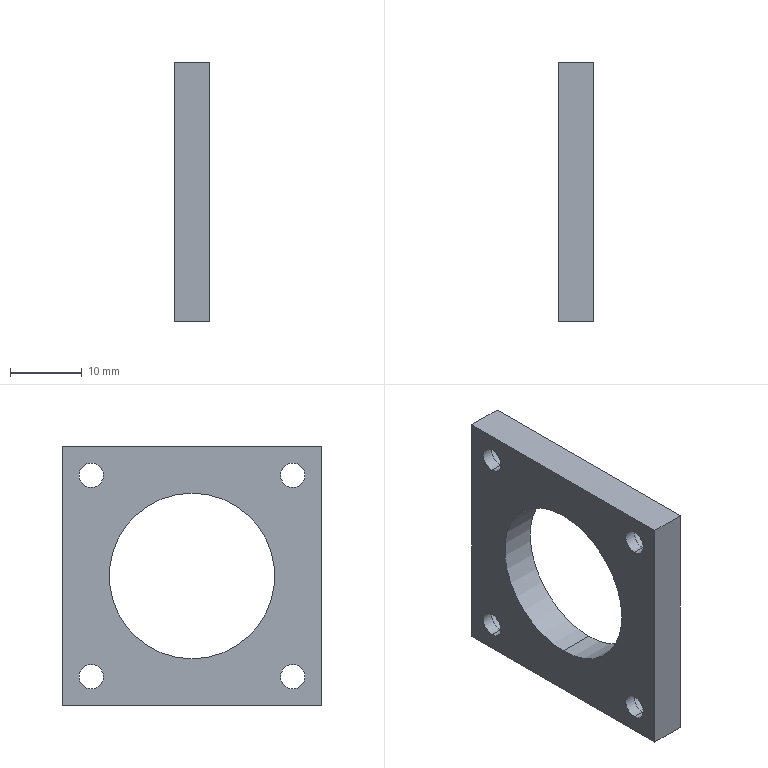Part | SolidWorks | features Extrusion 1, HoleWzd 1, ICE 1 | 1 solid | 28 faces | box 5 x 36 x 36 mm | volume 3893 mm3 | cylinder 18 | plane 10 | commonest cylinder face diameters 3.4 x8 6.5 x8 23 x2
STEP:
#1=CARTESIAN_POINT('',(-2.5,0.,11.5));
#2=VERTEX_POINT('',#1);
#3=CARTESIAN_POINT('',(-2.5,0.,-11.5));
#4=VERTEX_POINT('',#3);
#5=CARTESIAN_POINT('',(-2.5,0.,0.));
#6=DIRECTION('',(1.,0.,0.));
#7=DIRECTION('',(0.,0.,-1.));
#8=AXIS2_PLACEMENT_3D('',#5,#6,#7);
#9=CIRCLE('',#8,11.5);
#10=EDGE_CURVE('',#2,#4,#9,.T.);
#11=ORIENTED_EDGE('',*,*,#10,.F.);
#12=CARTESIAN_POINT('',(2.5,0.,11.5));
#13=VERTEX_POINT('',#12);
#14=CARTESIAN_POINT('',(-2.5,0.,11.5));
#15=DIRECTION('',(1.,0.,0.));
#16=VECTOR('',#15,1000.);
#17=LINE('',#14,#16);
#18=EDGE_CURVE('',#2,#13,#17,.T.);
#19=ORIENTED_EDGE('',*,*,#18,.T.);
#20=CARTESIAN_POINT('',(2.5,0.,-11.5));
#21=VERTEX_POINT('',#20);
#22=CARTESIAN_POINT('',(2.5,0.,0.));
#23=DIRECTION('',(1.,0.,0.));
#24=DIRECTION('',(0.,0.,-1.));
#25=AXIS2_PLACEMENT_3D('',#22,#23,#24);
#26=CIRCLE('',#25,11.5);
#27=EDGE_CURVE('',#13,#21,#26,.T.);
#28=ORIENTED_EDGE('',*,*,#27,.T.);
#29=CARTESIAN_POINT('',(-2.5,0.,-11.5));
#30=DIRECTION('',(1.,0.,0.));
#31=VECTOR('',#30,1000.);
#32=LINE('',#29,#31);
#33=EDGE_CURVE('',#4,#21,#32,.T.);
#34=ORIENTED_EDGE('',*,*,#33,.F.);
#35=EDGE_LOOP('',(#11,#19,#28,#34));
#36=FACE_OUTER_BOUND('',#35,.T.);
#37=CARTESIAN_POINT('',(-2.5,0.,0.));
#38=DIRECTION('',(1.,0.,0.));
#39=DIRECTION('',(0.,0.,-1.));
#40=AXIS2_PLACEMENT_3D('',#37,#38,#39);
#41=CYLINDRICAL_SURFACE('',#40,11.5);
#42=ADVANCED_FACE('',(#36),#41,.F.);
#43=CARTESIAN_POINT('',(-0.9,14.,17.25));
#44=VERTEX_POINT('',#43);
#45=CARTESIAN_POINT('',(-0.9,14.,10.75));
#46=VERTEX_POINT('',#45);
#47=CARTESIAN_POINT('',(-0.9,14.,14.));
#48=DIRECTION('',(1.,0.,0.));
#49=DIRECTION('',(0.,0.,-1.));
#50=AXIS2_PLACEMENT_3D('',#47,#48,#49);
#51=CIRCLE('',#50,3.25);
#52=EDGE_CURVE('',#44,#46,#51,.T.);
#53=ORIENTED_EDGE('',*,*,#52,.F.);
#54=CARTESIAN_POINT('',(2.5,14.,17.25));
#55=VERTEX_POINT('',#54);
#56=CARTESIAN_POINT('',(2.5,14.,17.25));
#57=DIRECTION('',(1.,0.,0.));
#58=VECTOR('',#57,1000.);
#59=LINE('',#56,#58);
#60=EDGE_CURVE('',#44,#55,#59,.T.);
#61=ORIENTED_EDGE('',*,*,#60,.T.);
#62=CARTESIAN_POINT('',(2.5,14.,10.75));
#63=VERTEX_POINT('',#62);
#64=CARTESIAN_POINT('',(2.5,14.,14.));
#65=DIRECTION('',(1.,0.,0.));
#66=DIRECTION('',(0.,0.,-1.));
#67=AXIS2_PLACEMENT_3D('',#64,#65,#66);
#68=CIRCLE('',#67,3.25);
#69=EDGE_CURVE('',#55,#63,#68,.T.);
#70=ORIENTED_EDGE('',*,*,#69,.T.);
#71=CARTESIAN_POINT('',(2.5,14.,10.75));
#72=DIRECTION('',(1.,0.,0.));
#73=VECTOR('',#72,1000.);
#74=LINE('',#71,#73);
#75=EDGE_CURVE('',#46,#63,#74,.T.);
#76=ORIENTED_EDGE('',*,*,#75,.F.);
#77=EDGE_LOOP('',(#53,#61,#70,#76));
#78=FACE_OUTER_BOUND('',#77,.T.);
#79=CARTESIAN_POINT('',(2.5,14.,14.));
#80=DIRECTION('',(1.,0.,0.));
#81=DIRECTION('',(0.,0.,-1.));
#82=AXIS2_PLACEMENT_3D('',#79,#80,#81);
#83=CYLINDRICAL_SURFACE('',#82,3.25);
#84=ADVANCED_FACE('',(#78),#83,.F.);
#85=CARTESIAN_POINT('',(-2.5,14.,15.7));
#86=VERTEX_POINT('',#85);
#87=CARTESIAN_POINT('',(-2.5,14.,12.3));
#88=VERTEX_POINT('',#87);
#89=CARTESIAN_POINT('',(-2.5,14.,14.));
#90=DIRECTION('',(1.,0.,0.));
#91=DIRECTION('',(0.,0.,-1.));
#92=AXIS2_PLACEMENT_3D('',#89,#90,#91);
#93=CIRCLE('',#92,1.7);
#94=EDGE_CURVE('',#86,#88,#93,.T.);
#95=ORIENTED_EDGE('',*,*,#94,.F.);
#96=CARTESIAN_POINT('',(-0.9,14.,15.7));
#97=VERTEX_POINT('',#96);
#98=CARTESIAN_POINT('',(2.5,14.,15.7));
#99=DIRECTION('',(1.,0.,0.));
#100=VECTOR('',#99,1000.);
#101=LINE('',#98,#100);
#102=EDGE_CURVE('',#86,#97,#101,.T.);
#103=ORIENTED_EDGE('',*,*,#102,.T.);
#104=CARTESIAN_POINT('',(-0.9,14.,12.3));
#105=VERTEX_POINT('',#104);
#106=CARTESIAN_POINT('',(-0.9,14.,14.));
#107=DIRECTION('',(1.,0.,0.));
#108=DIRECTION('',(0.,0.,-1.));
#109=AXIS2_PLACEMENT_3D('',#106,#107,#108);
#110=CIRCLE('',#109,1.7);
#111=EDGE_CURVE('',#97,#105,#110,.T.);
#112=ORIENTED_EDGE('',*,*,#111,.T.);
#113=CARTESIAN_POINT('',(2.5,14.,12.3));
#114=DIRECTION('',(1.,0.,0.));
#115=VECTOR('',#114,1000.);
#116=LINE('',#113,#115);
#117=EDGE_CURVE('',#88,#105,#116,.T.);
#118=ORIENTED_EDGE('',*,*,#117,.F.);
#119=EDGE_LOOP('',(#95,#103,#112,#118));
#120=FACE_OUTER_BOUND('',#119,.T.);
#121=CARTESIAN_POINT('',(2.5,14.,14.));
#122=DIRECTION('',(1.,0.,0.));
#123=DIRECTION('',(0.,0.,-1.));
#124=AXIS2_PLACEMENT_3D('',#121,#122,#123);
#125=CYLINDRICAL_SURFACE('',#124,1.7);
#126=ADVANCED_FACE('',(#120),#125,.F.);
#127=CARTESIAN_POINT('',(-0.9,14.,-10.75));
#128=VERTEX_POINT('',#127);
#129=CARTESIAN_POINT('',(-0.9,14.,-17.25));
#130=VERTEX_POINT('',#129);
#131=CARTESIAN_POINT('',(-0.9,14.,-14.));
#132=DIRECTION('',(1.,0.,0.));
#133=DIRECTION('',(0.,0.,-1.));
#134=AXIS2_PLACEMENT_3D('',#131,#132,#133);
#135=CIRCLE('',#134,3.25);
#136=EDGE_CURVE('',#128,#130,#135,.T.);
#137=ORIENTED_EDGE('',*,*,#136,.F.);
#138=CARTESIAN_POINT('',(2.5,14.,-10.75));
#139=VERTEX_POINT('',#138);
#140=CARTESIAN_POINT('',(2.5,14.,-10.75));
#141=DIRECTION('',(1.,0.,0.));
#142=VECTOR('',#141,1000.);
#143=LINE('',#140,#142);
#144=EDGE_CURVE('',#128,#139,#143,.T.);
#145=ORIENTED_EDGE('',*,*,#144,.T.);
#146=CARTESIAN_POINT('',(2.5,14.,-17.25));
#147=VERTEX_POINT('',#146);
#148=CARTESIAN_POINT('',(2.5,14.,-14.));
#149=DIRECTION('',(1.,0.,0.));
#150=DIRECTION('',(0.,0.,-1.));
#151=AXIS2_PLACEMENT_3D('',#148,#149,#150);
#152=CIRCLE('',#151,3.25);
#153=EDGE_CURVE('',#139,#147,#152,.T.);
#154=ORIENTED_EDGE('',*,*,#153,.T.);
#155=CARTESIAN_POINT('',(2.5,14.,-17.25));
#156=DIRECTION('',(1.,0.,0.));
#157=VECTOR('',#156,1000.);
#158=LINE('',#155,#157);
#159=EDGE_CURVE('',#130,#147,#158,.T.);
#160=ORIENTED_EDGE('',*,*,#159,.F.);
#161=EDGE_LOOP('',(#137,#145,#154,#160));
#162=FACE_OUTER_BOUND('',#161,.T.);
#163=CARTESIAN_POINT('',(2.5,14.,-14.));
#164=DIRECTION('',(1.,0.,0.));
#165=DIRECTION('',(0.,0.,-1.));
#166=AXIS2_PLACEMENT_3D('',#163,#164,#165);
#167=CYLINDRICAL_SURFACE('',#166,3.25);
#168=ADVANCED_FACE('',(#162),#167,.F.);
#169=CARTESIAN_POINT('',(-2.5,14.,-12.3));
#170=VERTEX_POINT('',#169);
#171=CARTESIAN_POINT('',(-2.5,14.,-15.7));
#172=VERTEX_POINT('',#171);
#173=CARTESIAN_POINT('',(-2.5,14.,-14.));
#174=DIRECTION('',(1.,0.,0.));
#175=DIRECTION('',(0.,0.,-1.));
#176=AXIS2_PLACEMENT_3D('',#173,#174,#175);
#177=CIRCLE('',#176,1.7);
#178=EDGE_CURVE('',#170,#172,#177,.T.);
#179=ORIENTED_EDGE('',*,*,#178,.F.);
#180=CARTESIAN_POINT('',(-0.9,14.,-12.3));
#181=VERTEX_POINT('',#180);
#182=CARTESIAN_POINT('',(2.5,14.,-12.3));
#183=DIRECTION('',(1.,0.,0.));
#184=VECTOR('',#183,1000.);
#185=LINE('',#182,#184);
#186=EDGE_CURVE('',#170,#181,#185,.T.);
#187=ORIENTED_EDGE('',*,*,#186,.T.);
#188=CARTESIAN_POINT('',(-0.9,14.,-15.7));
#189=VERTEX_POINT('',#188);
#190=CARTESIAN_POINT('',(-0.9,14.,-14.));
#191=DIRECTION('',(1.,0.,0.));
#192=DIRECTION('',(0.,0.,-1.));
#193=AXIS2_PLACEMENT_3D('',#190,#191,#192);
#194=CIRCLE('',#193,1.7);
#195=EDGE_CURVE('',#181,#189,#194,.T.);
#196=ORIENTED_EDGE('',*,*,#195,.T.);
#197=CARTESIAN_POINT('',(2.5,14.,-15.7));
#198=DIRECTION('',(1.,0.,0.));
#199=VECTOR('',#198,1000.);
#200=LINE('',#197,#199);
#201=EDGE_CURVE('',#172,#189,#200,.T.);
#202=ORIENTED_EDGE('',*,*,#201,.F.);
#203=EDGE_LOOP('',(#179,#187,#196,#202));
#204=FACE_OUTER_BOUND('',#203,.T.);
#205=CARTESIAN_POINT('',(2.5,14.,-14.));
#206=DIRECTION('',(1.,0.,0.));
#207=DIRECTION('',(0.,0.,-1.));
#208=AXIS2_PLACEMENT_3D('',#205,#206,#207);
#209=CYLINDRICAL_SURFACE('',#208,1.7);
#210=ADVANCED_FACE('',(#204),#209,.F.);
#211=CARTESIAN_POINT('',(-0.9,-14.,17.25));
#212=VERTEX_POINT('',#211);
#213=CARTESIAN_POINT('',(-0.9,-14.,10.75));
#214=VERTEX_POINT('',#213);
#215=CARTESIAN_POINT('',(-0.9,-14.,14.));
#216=DIRECTION('',(1.,0.,0.));
#217=DIRECTION('',(0.,0.,-1.));
#218=AXIS2_PLACEMENT_3D('',#215,#216,#217);
#219=CIRCLE('',#218,3.25);
#220=EDGE_CURVE('',#212,#214,#219,.T.);
#221=ORIENTED_EDGE('',*,*,#220,.F.);
#222=CARTESIAN_POINT('',(2.5,-14.,17.25));
#223=VERTEX_POINT('',#222);
#224=CARTESIAN_POINT('',(2.5,-14.,17.25));
#225=DIRECTION('',(1.,0.,0.));
#226=VECTOR('',#225,1000.);
#227=LINE('',#224,#226);
#228=EDGE_CURVE('',#212,#223,#227,.T.);
#229=ORIENTED_EDGE('',*,*,#228,.T.);
#230=CARTESIAN_POINT('',(2.5,-14.,10.75));
#231=VERTEX_POINT('',#230);
#232=CARTESIAN_POINT('',(2.5,-14.,14.));
#233=DIRECTION('',(1.,0.,0.));
#234=DIRECTION('',(0.,0.,-1.));
#235=AXIS2_PLACEMENT_3D('',#232,#233,#234);
#236=CIRCLE('',#235,3.25);
#237=EDGE_CURVE('',#223,#231,#236,.T.);
#238=ORIENTED_EDGE('',*,*,#237,.T.);
#239=CARTESIAN_POINT('',(2.5,-14.,10.75));
#240=DIRECTION('',(1.,0.,0.));
#241=VECTOR('',#240,1000.);
#242=LINE('',#239,#241);
#243=EDGE_CURVE('',#214,#231,#242,.T.);
#244=ORIENTED_EDGE('',*,*,#243,.F.);
#245=EDGE_LOOP('',(#221,#229,#238,#244));
#246=FACE_OUTER_BOUND('',#245,.T.);
#247=CARTESIAN_POINT('',(2.5,-14.,14.));
#248=DIRECTION('',(1.,0.,0.));
#249=DIRECTION('',(0.,0.,-1.));
#250=AXIS2_PLACEMENT_3D('',#247,#248,#249);
#251=CYLINDRICAL_SURFACE('',#250,3.25);
#252=ADVANCED_FACE('',(#246),#251,.F.);
#253=CARTESIAN_POINT('',(-2.5,-14.,15.7));
#254=VERTEX_POINT('',#253);
#255=CARTESIAN_POINT('',(-2.5,-14.,12.3));
#256=VERTEX_POINT('',#255);
#257=CARTESIAN_POINT('',(-2.5,-14.,14.));
#258=DIRECTION('',(1.,0.,0.));
#259=DIRECTION('',(0.,0.,-1.));
#260=AXIS2_PLACEMENT_3D('',#257,#258,#259);
#261=CIRCLE('',#260,1.7);
#262=EDGE_CURVE('',#254,#256,#261,.T.);
#263=ORIENTED_EDGE('',*,*,#262,.F.);
#264=CARTESIAN_POINT('',(-0.9,-14.,15.7));
#265=VERTEX_POINT('',#264);
#266=CARTESIAN_POINT('',(2.5,-14.,15.7));
#267=DIRECTION('',(1.,0.,0.));
#268=VECTOR('',#267,1000.);
#269=LINE('',#266,#268);
#270=EDGE_CURVE('',#254,#265,#269,.T.);
#271=ORIENTED_EDGE('',*,*,#270,.T.);
#272=CARTESIAN_POINT('',(-0.9,-14.,12.3));
#273=VERTEX_POINT('',#272);
#274=CARTESIAN_POINT('',(-0.9,-14.,14.));
#275=DIRECTION('',(1.,0.,0.));
#276=DIRECTION('',(0.,0.,-1.));
#277=AXIS2_PLACEMENT_3D('',#274,#275,#276);
#278=CIRCLE('',#277,1.7);
#279=EDGE_CURVE('',#265,#273,#278,.T.);
#280=ORIENTED_EDGE('',*,*,#279,.T.);
#281=CARTESIAN_POINT('',(2.5,-14.,12.3));
#282=DIRECTION('',(1.,0.,0.));
#283=VECTOR('',#282,1000.);
#284=LINE('',#281,#283);
#285=EDGE_CURVE('',#256,#273,#284,.T.);
#286=ORIENTED_EDGE('',*,*,#285,.F.);
#287=EDGE_LOOP('',(#263,#271,#280,#286));
#288=FACE_OUTER_BOUND('',#287,.T.);
#289=CARTESIAN_POINT('',(2.5,-14.,14.));
#290=DIRECTION('',(1.,0.,0.));
#291=DIRECTION('',(0.,0.,-1.));
#292=AXIS2_PLACEMENT_3D('',#289,#290,#291);
#293=CYLINDRICAL_SURFACE('',#292,1.7);
#294=ADVANCED_FACE('',(#288),#293,.F.);
#295=CARTESIAN_POINT('',(-0.9,-14.,-10.75));
#296=VERTEX_POINT('',#295);
#297=CARTESIAN_POINT('',(-0.9,-14.,-17.25));
#298=VERTEX_POINT('',#297);
#299=CARTESIAN_POINT('',(-0.9,-14.,-14.));
#300=DIRECTION('',(1.,0.,0.));
#301=DIRECTION('',(0.,0.,-1.));
#302=AXIS2_PLACEMENT_3D('',#299,#300,#301);
#303=CIRCLE('',#302,3.25);
#304=EDGE_CURVE('',#296,#298,#303,.T.);
#305=ORIENTED_EDGE('',*,*,#304,.F.);
#306=CARTESIAN_POINT('',(2.5,-14.,-10.75));
#307=VERTEX_POINT('',#306);
#308=CARTESIAN_POINT('',(2.5,-14.,-10.75));
#309=DIRECTION('',(1.,0.,0.));
#310=VECTOR('',#309,1000.);
#311=LINE('',#308,#310);
#312=EDGE_CURVE('',#296,#307,#311,.T.);
#313=ORIENTED_EDGE('',*,*,#312,.T.);
#314=CARTESIAN_POINT('',(2.5,-14.,-17.25));
#315=VERTEX_POINT('',#314);
#316=CARTESIAN_POINT('',(2.5,-14.,-14.));
#317=DIRECTION('',(1.,0.,0.));
#318=DIRECTION('',(0.,0.,-1.));
#319=AXIS2_PLACEMENT_3D('',#316,#317,#318);
#320=CIRCLE('',#319,3.25);
#321=EDGE_CURVE('',#307,#315,#320,.T.);
#322=ORIENTED_EDGE('',*,*,#321,.T.);
#323=CARTESIAN_POINT('',(2.5,-14.,-17.25));
#324=DIRECTION('',(1.,0.,0.));
#325=VECTOR('',#324,1000.);
#326=LINE('',#323,#325);
#327=EDGE_CURVE('',#298,#315,#326,.T.);
#328=ORIENTED_EDGE('',*,*,#327,.F.);
#329=EDGE_LOOP('',(#305,#313,#322,#328));
#330=FACE_OUTER_BOUND('',#329,.T.);
#331=CARTESIAN_POINT('',(2.5,-14.,-14.));
#332=DIRECTION('',(1.,0.,0.));
#333=DIRECTION('',(0.,0.,-1.));
#334=AXIS2_PLACEMENT_3D('',#331,#332,#333);
#335=CYLINDRICAL_SURFACE('',#334,3.25);
#336=ADVANCED_FACE('',(#330),#335,.F.);
#337=CARTESIAN_POINT('',(-2.5,-14.,-12.3));
#338=VERTEX_POINT('',#337);
#339=CARTESIAN_POINT('',(-2.5,-14.,-15.7));
#340=VERTEX_POINT('',#339);
#341=CARTESIAN_POINT('',(-2.5,-14.,-14.));
#342=DIRECTION('',(1.,0.,0.));
#343=DIRECTION('',(0.,0.,-1.));
#344=AXIS2_PLACEMENT_3D('',#341,#342,#343);
#345=CIRCLE('',#344,1.7);
#346=EDGE_CURVE('',#338,#340,#345,.T.);
#347=ORIENTED_EDGE('',*,*,#346,.F.);
#348=CARTESIAN_POINT('',(-0.9,-14.,-12.3));
#349=VERTEX_POINT('',#348);
#350=CARTESIAN_POINT('',(2.5,-14.,-12.3));
#351=DIRECTION('',(1.,0.,0.));
#352=VECTOR('',#351,1000.);
#353=LINE('',#350,#352);
#354=EDGE_CURVE('',#338,#349,#353,.T.);
#355=ORIENTED_EDGE('',*,*,#354,.T.);
#356=CARTESIAN_POINT('',(-0.9,-14.,-15.7));
#357=VERTEX_POINT('',#356);
#358=CARTESIAN_POINT('',(-0.9,-14.,-14.));
#359=DIRECTION('',(1.,0.,0.));
#360=DIRECTION('',(0.,0.,-1.));
#361=AXIS2_PLACEMENT_3D('',#358,#359,#360);
#362=CIRCLE('',#361,1.7);
#363=EDGE_CURVE('',#349,#357,#362,.T.);
#364=ORIENTED_EDGE('',*,*,#363,.T.);
#365=CARTESIAN_POINT('',(2.5,-14.,-15.7));
#366=DIRECTION('',(1.,0.,0.));
#367=VECTOR('',#366,1000.);
#368=LINE('',#365,#367);
#369=EDGE_CURVE('',#340,#357,#368,.T.);
#370=ORIENTED_EDGE('',*,*,#369,.F.);
#371=EDGE_LOOP('',(#347,#355,#364,#370));
#372=FACE_OUTER_BOUND('',#371,.T.);
#373=CARTESIAN_POINT('',(2.5,-14.,-14.));
#374=DIRECTION('',(1.,0.,0.));
#375=DIRECTION('',(0.,0.,-1.));
#376=AXIS2_PLACEMENT_3D('',#373,#374,#375);
#377=CYLINDRICAL_SURFACE('',#376,1.7);
#378=ADVANCED_FACE('',(#372),#377,.F.);
#379=CARTESIAN_POINT('',(-2.5,-18.,-18.));
#380=VERTEX_POINT('',#379);
#381=CARTESIAN_POINT('',(-2.5,18.,-18.));
#382=VERTEX_POINT('',#381);
#383=CARTESIAN_POINT('',(-2.5,18.,-18.));
#384=DIRECTION('',(0.,1.,0.));
#385=VECTOR('',#384,1000.);
#386=LINE('',#383,#385);
#387=EDGE_CURVE('',#380,#382,#386,.T.);
#388=ORIENTED_EDGE('',*,*,#387,.T.);
#389=CARTESIAN_POINT('',(2.5,18.,-18.));
#390=VERTEX_POINT('',#389);
#391=CARTESIAN_POINT('',(2.5,18.,-18.));
#392=DIRECTION('',(-1.,0.,0.));
#393=VECTOR('',#392,1000.);
#394=LINE('',#391,#393);
#395=EDGE_CURVE('',#390,#382,#394,.T.);
#396=ORIENTED_EDGE('',*,*,#395,.F.);
#397=CARTESIAN_POINT('',(2.5,-18.,-18.));
#398=VERTEX_POINT('',#397);
#399=CARTESIAN_POINT('',(2.5,18.,-18.));
#400=DIRECTION('',(0.,1.,0.));
#401=VECTOR('',#400,1000.);
#402=LINE('',#399,#401);
#403=EDGE_CURVE('',#398,#390,#402,.T.);
#404=ORIENTED_EDGE('',*,*,#403,.F.);
#405=CARTESIAN_POINT('',(2.5,-18.,-18.));
#406=DIRECTION('',(-1.,0.,0.));
#407=VECTOR('',#406,1000.);
#408=LINE('',#405,#407);
#409=EDGE_CURVE('',#398,#380,#408,.T.);
#410=ORIENTED_EDGE('',*,*,#409,.T.);
#411=EDGE_LOOP('',(#388,#396,#404,#410));
#412=FACE_OUTER_BOUND('',#411,.T.);
#413=CARTESIAN_POINT('',(2.5,18.,-18.));
#414=DIRECTION('',(0.,0.,1.));
#415=DIRECTION('',(0.,-1.,0.));
#416=AXIS2_PLACEMENT_3D('',#413,#414,#415);
#417=PLANE('',#416);
#418=ADVANCED_FACE('',(#412),#417,.F.);
#419=CARTESIAN_POINT('',(-2.5,18.,18.));
#420=VERTEX_POINT('',#419);
#421=CARTESIAN_POINT('',(-2.5,18.,18.));
#422=DIRECTION('',(0.,0.,1.));
#423=VECTOR('',#422,1000.);
#424=LINE('',#421,#423);
#425=EDGE_CURVE('',#382,#420,#424,.T.);
#426=ORIENTED_EDGE('',*,*,#425,.T.);
#427=CARTESIAN_POINT('',(2.5,18.,18.));
#428=VERTEX_POINT('',#427);
#429=CARTESIAN_POINT('',(2.5,18.,18.));
#430=DIRECTION('',(-1.,0.,0.));
#431=VECTOR('',#430,1000.);
#432=LINE('',#429,#431);
#433=EDGE_CURVE('',#428,#420,#432,.T.);
#434=ORIENTED_EDGE('',*,*,#433,.F.);
#435=CARTESIAN_POINT('',(2.5,18.,18.));
#436=DIRECTION('',(0.,0.,1.));
#437=VECTOR('',#436,1000.);
#438=LINE('',#435,#437);
#439=EDGE_CURVE('',#390,#428,#438,.T.);
#440=ORIENTED_EDGE('',*,*,#439,.F.);
#441=ORIENTED_EDGE('',*,*,#395,.T.);
#442=EDGE_LOOP('',(#426,#434,#440,#441));
#443=FACE_OUTER_BOUND('',#442,.T.);
#444=CARTESIAN_POINT('',(2.5,18.,18.));
#445=DIRECTION('',(0.,-1.,0.));
#446=DIRECTION('',(0.,0.,-1.));
#447=AXIS2_PLACEMENT_3D('',#444,#445,#446);
#448=PLANE('',#447);
#449=ADVANCED_FACE('',(#443),#448,.F.);
#450=CARTESIAN_POINT('',(-2.5,-18.,18.));
#451=VERTEX_POINT('',#450);
#452=CARTESIAN_POINT('',(-2.5,18.,18.));
#453=DIRECTION('',(0.,-1.,0.));
#454=VECTOR('',#453,1000.);
#455=LINE('',#452,#454);
#456=EDGE_CURVE('',#420,#451,#455,.T.);
#457=ORIENTED_EDGE('',*,*,#456,.T.);
#458=CARTESIAN_POINT('',(2.5,-18.,18.));
#459=VERTEX_POINT('',#458);
#460=CARTESIAN_POINT('',(2.5,-18.,18.));
#461=DIRECTION('',(-1.,0.,0.));
#462=VECTOR('',#461,1000.);
#463=LINE('',#460,#462);
#464=EDGE_CURVE('',#459,#451,#463,.T.);
#465=ORIENTED_EDGE('',*,*,#464,.F.);
#466=CARTESIAN_POINT('',(2.5,18.,18.));
#467=DIRECTION('',(0.,-1.,0.));
#468=VECTOR('',#467,1000.);
#469=LINE('',#466,#468);
#470=EDGE_CURVE('',#428,#459,#469,.T.);
#471=ORIENTED_EDGE('',*,*,#470,.F.);
#472=ORIENTED_EDGE('',*,*,#433,.T.);
#473=EDGE_LOOP('',(#457,#465,#471,#472));
#474=FACE_OUTER_BOUND('',#473,.T.);
#475=CARTESIAN_POINT('',(2.5,18.,18.));
#476=DIRECTION('',(0.,0.,-1.));
#477=DIRECTION('',(0.,1.,0.));
#478=AXIS2_PLACEMENT_3D('',#475,#476,#477);
#479=PLANE('',#478);
#480=ADVANCED_FACE('',(#474),#479,.F.);
#481=CARTESIAN_POINT('',(-2.5,-18.,18.));
#482=DIRECTION('',(0.,0.,-1.));
#483=VECTOR('',#482,1000.);
#484=LINE('',#481,#483);
#485=EDGE_CURVE('',#451,#380,#484,.T.);
#486=ORIENTED_EDGE('',*,*,#485,.T.);
#487=ORIENTED_EDGE('',*,*,#409,.F.);
#488=CARTESIAN_POINT('',(2.5,-18.,18.));
#489=DIRECTION('',(0.,0.,-1.));
#490=VECTOR('',#489,1000.);
#491=LINE('',#488,#490);
#492=EDGE_CURVE('',#459,#398,#491,.T.);
#493=ORIENTED_EDGE('',*,*,#492,.F.);
#494=ORIENTED_EDGE('',*,*,#464,.T.);
#495=EDGE_LOOP('',(#486,#487,#493,#494));
#496=FACE_OUTER_BOUND('',#495,.T.);
#497=CARTESIAN_POINT('',(2.5,-18.,18.));
#498=DIRECTION('',(0.,1.,0.));
#499=DIRECTION('',(0.,0.,1.));
#500=AXIS2_PLACEMENT_3D('',#497,#498,#499);
#501=PLANE('',#500);
#502=ADVANCED_FACE('',(#496),#501,.F.);
#503=CARTESIAN_POINT('',(2.5,0.,0.));
#504=DIRECTION('',(1.,0.,0.));
#505=DIRECTION('',(0.,0.,-1.));
#506=AXIS2_PLACEMENT_3D('',#503,#504,#505);
#507=CIRCLE('',#506,11.5);
#508=EDGE_CURVE('',#21,#13,#507,.T.);
#509=ORIENTED_EDGE('',*,*,#508,.F.);
#510=ORIENTED_EDGE('',*,*,#27,.F.);
#511=EDGE_LOOP('',(#509,#510));
#512=FACE_BOUND('',#511,.T.);
#513=CARTESIAN_POINT('',(2.5,14.,14.));
#514=DIRECTION('',(1.,0.,0.));
#515=DIRECTION('',(0.,0.,-1.));
#516=AXIS2_PLACEMENT_3D('',#513,#514,#515);
#517=CIRCLE('',#516,3.25);
#518=EDGE_CURVE('',#63,#55,#517,.T.);
#519=ORIENTED_EDGE('',*,*,#518,.F.);
#520=ORIENTED_EDGE('',*,*,#69,.F.);
#521=EDGE_LOOP('',(#519,#520));
#522=FACE_BOUND('',#521,.T.);
#523=CARTESIAN_POINT('',(2.5,14.,-14.));
#524=DIRECTION('',(1.,0.,0.));
#525=DIRECTION('',(0.,0.,-1.));
#526=AXIS2_PLACEMENT_3D('',#523,#524,#525);
#527=CIRCLE('',#526,3.25);
#528=EDGE_CURVE('',#147,#139,#527,.T.);
#529=ORIENTED_EDGE('',*,*,#528,.F.);
#530=ORIENTED_EDGE('',*,*,#153,.F.);
#531=EDGE_LOOP('',(#529,#530));
#532=FACE_BOUND('',#531,.T.);
#533=CARTESIAN_POINT('',(2.5,-14.,14.));
#534=DIRECTION('',(1.,0.,0.));
#535=DIRECTION('',(0.,0.,-1.));
#536=AXIS2_PLACEMENT_3D('',#533,#534,#535);
#537=CIRCLE('',#536,3.25);
#538=EDGE_CURVE('',#231,#223,#537,.T.);
#539=ORIENTED_EDGE('',*,*,#538,.F.);
#540=ORIENTED_EDGE('',*,*,#237,.F.);
#541=EDGE_LOOP('',(#539,#540));
#542=FACE_BOUND('',#541,.T.);
#543=CARTESIAN_POINT('',(2.5,-14.,-14.));
#544=DIRECTION('',(1.,0.,0.));
#545=DIRECTION('',(0.,0.,-1.));
#546=AXIS2_PLACEMENT_3D('',#543,#544,#545);
#547=CIRCLE('',#546,3.25);
#548=EDGE_CURVE('',#315,#307,#547,.T.);
#549=ORIENTED_EDGE('',*,*,#548,.F.);
#550=ORIENTED_EDGE('',*,*,#321,.F.);
#551=EDGE_LOOP('',(#549,#550));
#552=FACE_BOUND('',#551,.T.);
#553=ORIENTED_EDGE('',*,*,#403,.T.);
#554=ORIENTED_EDGE('',*,*,#439,.T.);
#555=ORIENTED_EDGE('',*,*,#470,.T.);
#556=ORIENTED_EDGE('',*,*,#492,.T.);
#557=EDGE_LOOP('',(#553,#554,#555,#556));
#558=FACE_OUTER_BOUND('',#557,.T.);
#559=CARTESIAN_POINT('',(2.5,0.,0.));
#560=DIRECTION('',(1.,0.,0.));
#561=DIRECTION('',(0.,0.,-1.));
#562=AXIS2_PLACEMENT_3D('',#559,#560,#561);
#563=PLANE('',#562);
#564=ADVANCED_FACE('',(#512,#522,#532,#542,#552,#558),#563,.T.);
#565=CARTESIAN_POINT('',(-2.5,0.,0.));
#566=DIRECTION('',(1.,0.,0.));
#567=DIRECTION('',(0.,0.,-1.));
#568=AXIS2_PLACEMENT_3D('',#565,#566,#567);
#569=CIRCLE('',#568,11.5);
#570=EDGE_CURVE('',#4,#2,#569,.T.);
#571=ORIENTED_EDGE('',*,*,#570,.T.);
#572=ORIENTED_EDGE('',*,*,#10,.T.);
#573=EDGE_LOOP('',(#571,#572));
#574=FACE_BOUND('',#573,.T.);
#575=CARTESIAN_POINT('',(-2.5,14.,14.));
#576=DIRECTION('',(1.,0.,0.));
#577=DIRECTION('',(0.,0.,-1.));
#578=AXIS2_PLACEMENT_3D('',#575,#576,#577);
#579=CIRCLE('',#578,1.7);
#580=EDGE_CURVE('',#88,#86,#579,.T.);
#581=ORIENTED_EDGE('',*,*,#580,.T.);
#582=ORIENTED_EDGE('',*,*,#94,.T.);
#583=EDGE_LOOP('',(#581,#582));
#584=FACE_BOUND('',#583,.T.);
#585=CARTESIAN_POINT('',(-2.5,14.,-14.));
#586=DIRECTION('',(1.,0.,0.));
#587=DIRECTION('',(0.,0.,-1.));
#588=AXIS2_PLACEMENT_3D('',#585,#586,#587);
#589=CIRCLE('',#588,1.7);
#590=EDGE_CURVE('',#172,#170,#589,.T.);
#591=ORIENTED_EDGE('',*,*,#590,.T.);
#592=ORIENTED_EDGE('',*,*,#178,.T.);
#593=EDGE_LOOP('',(#591,#592));
#594=FACE_BOUND('',#593,.T.);
#595=CARTESIAN_POINT('',(-2.5,-14.,14.));
#596=DIRECTION('',(1.,0.,0.));
#597=DIRECTION('',(0.,0.,-1.));
#598=AXIS2_PLACEMENT_3D('',#595,#596,#597);
#599=CIRCLE('',#598,1.7);
#600=EDGE_CURVE('',#256,#254,#599,.T.);
#601=ORIENTED_EDGE('',*,*,#600,.T.);
#602=ORIENTED_EDGE('',*,*,#262,.T.);
#603=EDGE_LOOP('',(#601,#602));
#604=FACE_BOUND('',#603,.T.);
#605=CARTESIAN_POINT('',(-2.5,-14.,-14.));
#606=DIRECTION('',(1.,0.,0.));
#607=DIRECTION('',(0.,0.,-1.));
#608=AXIS2_PLACEMENT_3D('',#605,#606,#607);
#609=CIRCLE('',#608,1.7);
#610=EDGE_CURVE('',#340,#338,#609,.T.);
#611=ORIENTED_EDGE('',*,*,#610,.T.);
#612=ORIENTED_EDGE('',*,*,#346,.T.);
#613=EDGE_LOOP('',(#611,#612));
#614=FACE_BOUND('',#613,.T.);
#615=ORIENTED_EDGE('',*,*,#387,.F.);
#616=ORIENTED_EDGE('',*,*,#485,.F.);
#617=ORIENTED_EDGE('',*,*,#456,.F.);
#618=ORIENTED_EDGE('',*,*,#425,.F.);
#619=EDGE_LOOP('',(#615,#616,#617,#618));
#620=FACE_OUTER_BOUND('',#619,.T.);
#621=CARTESIAN_POINT('',(-2.5,0.,0.));
#622=DIRECTION('',(1.,0.,0.));
#623=DIRECTION('',(0.,0.,-1.));
#624=AXIS2_PLACEMENT_3D('',#621,#622,#623);
#625=PLANE('',#624);
#626=ADVANCED_FACE('',(#574,#584,#594,#604,#614,#620),#625,.F.);
#627=ORIENTED_EDGE('',*,*,#354,.F.);
#628=ORIENTED_EDGE('',*,*,#610,.F.);
#629=ORIENTED_EDGE('',*,*,#369,.T.);
#630=CARTESIAN_POINT('',(-0.9,-14.,-14.));
#631=DIRECTION('',(1.,0.,0.));
#632=DIRECTION('',(0.,0.,-1.));
#633=AXIS2_PLACEMENT_3D('',#630,#631,#632);
#634=CIRCLE('',#633,1.7);
#635=EDGE_CURVE('',#357,#349,#634,.T.);
#636=ORIENTED_EDGE('',*,*,#635,.T.);
#637=EDGE_LOOP('',(#627,#628,#629,#636));
#638=FACE_OUTER_BOUND('',#637,.T.);
#639=CARTESIAN_POINT('',(2.5,-14.,-14.));
#640=DIRECTION('',(1.,0.,0.));
#641=DIRECTION('',(0.,0.,-1.));
#642=AXIS2_PLACEMENT_3D('',#639,#640,#641);
#643=CYLINDRICAL_SURFACE('',#642,1.7);
#644=ADVANCED_FACE('',(#638),#643,.F.);
#645=ORIENTED_EDGE('',*,*,#635,.F.);
#646=ORIENTED_EDGE('',*,*,#363,.F.);
#647=EDGE_LOOP('',(#645,#646));
#648=FACE_BOUND('',#647,.T.);
#649=CARTESIAN_POINT('',(-0.9,-14.,-14.));
#650=DIRECTION('',(1.,0.,0.));
#651=DIRECTION('',(0.,0.,-1.));
#652=AXIS2_PLACEMENT_3D('',#649,#650,#651);
#653=CIRCLE('',#652,3.25);
#654=EDGE_CURVE('',#298,#296,#653,.T.);
#655=ORIENTED_EDGE('',*,*,#654,.T.);
#656=ORIENTED_EDGE('',*,*,#304,.T.);
#657=EDGE_LOOP('',(#655,#656));
#658=FACE_OUTER_BOUND('',#657,.T.);
#659=CARTESIAN_POINT('',(-0.9,-12.3,-14.));
#660=DIRECTION('',(-1.,0.,0.));
#661=DIRECTION('',(0.,0.,1.));
#662=AXIS2_PLACEMENT_3D('',#659,#660,#661);
#663=PLANE('',#662);
#664=ADVANCED_FACE('',(#648,#658),#663,.F.);
#665=ORIENTED_EDGE('',*,*,#312,.F.);
#666=ORIENTED_EDGE('',*,*,#654,.F.);
#667=ORIENTED_EDGE('',*,*,#327,.T.);
#668=ORIENTED_EDGE('',*,*,#548,.T.);
#669=EDGE_LOOP('',(#665,#666,#667,#668));
#670=FACE_OUTER_BOUND('',#669,.T.);
#671=CARTESIAN_POINT('',(2.5,-14.,-14.));
#672=DIRECTION('',(1.,0.,0.));
#673=DIRECTION('',(0.,0.,-1.));
#674=AXIS2_PLACEMENT_3D('',#671,#672,#673);
#675=CYLINDRICAL_SURFACE('',#674,3.25);
#676=ADVANCED_FACE('',(#670),#675,.F.);
#677=ORIENTED_EDGE('',*,*,#270,.F.);
#678=ORIENTED_EDGE('',*,*,#600,.F.);
#679=ORIENTED_EDGE('',*,*,#285,.T.);
#680=CARTESIAN_POINT('',(-0.9,-14.,14.));
#681=DIRECTION('',(1.,0.,0.));
#682=DIRECTION('',(0.,0.,-1.));
#683=AXIS2_PLACEMENT_3D('',#680,#681,#682);
#684=CIRCLE('',#683,1.7);
#685=EDGE_CURVE('',#273,#265,#684,.T.);
#686=ORIENTED_EDGE('',*,*,#685,.T.);
#687=EDGE_LOOP('',(#677,#678,#679,#686));
#688=FACE_OUTER_BOUND('',#687,.T.);
#689=CARTESIAN_POINT('',(2.5,-14.,14.));
#690=DIRECTION('',(1.,0.,0.));
#691=DIRECTION('',(0.,0.,-1.));
#692=AXIS2_PLACEMENT_3D('',#689,#690,#691);
#693=CYLINDRICAL_SURFACE('',#692,1.7);
#694=ADVANCED_FACE('',(#688),#693,.F.);
#695=ORIENTED_EDGE('',*,*,#685,.F.);
#696=ORIENTED_EDGE('',*,*,#279,.F.);
#697=EDGE_LOOP('',(#695,#696));
#698=FACE_BOUND('',#697,.T.);
#699=CARTESIAN_POINT('',(-0.9,-14.,14.));
#700=DIRECTION('',(1.,0.,0.));
#701=DIRECTION('',(0.,0.,-1.));
#702=AXIS2_PLACEMENT_3D('',#699,#700,#701);
#703=CIRCLE('',#702,3.25);
#704=EDGE_CURVE('',#214,#212,#703,.T.);
#705=ORIENTED_EDGE('',*,*,#704,.T.);
#706=ORIENTED_EDGE('',*,*,#220,.T.);
#707=EDGE_LOOP('',(#705,#706));
#708=FACE_OUTER_BOUND('',#707,.T.);
#709=CARTESIAN_POINT('',(-0.9,-12.3,14.));
#710=DIRECTION('',(-1.,0.,0.));
#711=DIRECTION('',(0.,0.,1.));
#712=AXIS2_PLACEMENT_3D('',#709,#710,#711);
#713=PLANE('',#712);
#714=ADVANCED_FACE('',(#698,#708),#713,.F.);
#715=ORIENTED_EDGE('',*,*,#228,.F.);
#716=ORIENTED_EDGE('',*,*,#704,.F.);
#717=ORIENTED_EDGE('',*,*,#243,.T.);
#718=ORIENTED_EDGE('',*,*,#538,.T.);
#719=EDGE_LOOP('',(#715,#716,#717,#718));
#720=FACE_OUTER_BOUND('',#719,.T.);
#721=CARTESIAN_POINT('',(2.5,-14.,14.));
#722=DIRECTION('',(1.,0.,0.));
#723=DIRECTION('',(0.,0.,-1.));
#724=AXIS2_PLACEMENT_3D('',#721,#722,#723);
#725=CYLINDRICAL_SURFACE('',#724,3.25);
#726=ADVANCED_FACE('',(#720),#725,.F.);
#727=ORIENTED_EDGE('',*,*,#186,.F.);
#728=ORIENTED_EDGE('',*,*,#590,.F.);
#729=ORIENTED_EDGE('',*,*,#201,.T.);
#730=CARTESIAN_POINT('',(-0.9,14.,-14.));
#731=DIRECTION('',(1.,0.,0.));
#732=DIRECTION('',(0.,0.,-1.));
#733=AXIS2_PLACEMENT_3D('',#730,#731,#732);
#734=CIRCLE('',#733,1.7);
#735=EDGE_CURVE('',#189,#181,#734,.T.);
#736=ORIENTED_EDGE('',*,*,#735,.T.);
#737=EDGE_LOOP('',(#727,#728,#729,#736));
#738=FACE_OUTER_BOUND('',#737,.T.);
#739=CARTESIAN_POINT('',(2.5,14.,-14.));
#740=DIRECTION('',(1.,0.,0.));
#741=DIRECTION('',(0.,0.,-1.));
#742=AXIS2_PLACEMENT_3D('',#739,#740,#741);
#743=CYLINDRICAL_SURFACE('',#742,1.7);
#744=ADVANCED_FACE('',(#738),#743,.F.);
#745=ORIENTED_EDGE('',*,*,#735,.F.);
#746=ORIENTED_EDGE('',*,*,#195,.F.);
#747=EDGE_LOOP('',(#745,#746));
#748=FACE_BOUND('',#747,.T.);
#749=CARTESIAN_POINT('',(-0.9,14.,-14.));
#750=DIRECTION('',(1.,0.,0.));
#751=DIRECTION('',(0.,0.,-1.));
#752=AXIS2_PLACEMENT_3D('',#749,#750,#751);
#753=CIRCLE('',#752,3.25);
#754=EDGE_CURVE('',#130,#128,#753,.T.);
#755=ORIENTED_EDGE('',*,*,#754,.T.);
#756=ORIENTED_EDGE('',*,*,#136,.T.);
#757=EDGE_LOOP('',(#755,#756));
#758=FACE_OUTER_BOUND('',#757,.T.);
#759=CARTESIAN_POINT('',(-0.9,15.7,-14.));
#760=DIRECTION('',(-1.,0.,0.));
#761=DIRECTION('',(0.,0.,1.));
#762=AXIS2_PLACEMENT_3D('',#759,#760,#761);
#763=PLANE('',#762);
#764=ADVANCED_FACE('',(#748,#758),#763,.F.);
#765=ORIENTED_EDGE('',*,*,#144,.F.);
#766=ORIENTED_EDGE('',*,*,#754,.F.);
#767=ORIENTED_EDGE('',*,*,#159,.T.);
#768=ORIENTED_EDGE('',*,*,#528,.T.);
#769=EDGE_LOOP('',(#765,#766,#767,#768));
#770=FACE_OUTER_BOUND('',#769,.T.);
#771=CARTESIAN_POINT('',(2.5,14.,-14.));
#772=DIRECTION('',(1.,0.,0.));
#773=DIRECTION('',(0.,0.,-1.));
#774=AXIS2_PLACEMENT_3D('',#771,#772,#773);
#775=CYLINDRICAL_SURFACE('',#774,3.25);
#776=ADVANCED_FACE('',(#770),#775,.F.);
#777=ORIENTED_EDGE('',*,*,#102,.F.);
#778=ORIENTED_EDGE('',*,*,#580,.F.);
#779=ORIENTED_EDGE('',*,*,#117,.T.);
#780=CARTESIAN_POINT('',(-0.9,14.,14.));
#781=DIRECTION('',(1.,0.,0.));
#782=DIRECTION('',(0.,0.,-1.));
#783=AXIS2_PLACEMENT_3D('',#780,#781,#782);
#784=CIRCLE('',#783,1.7);
#785=EDGE_CURVE('',#105,#97,#784,.T.);
#786=ORIENTED_EDGE('',*,*,#785,.T.);
#787=EDGE_LOOP('',(#777,#778,#779,#786));
#788=FACE_OUTER_BOUND('',#787,.T.);
#789=CARTESIAN_POINT('',(2.5,14.,14.));
#790=DIRECTION('',(1.,0.,0.));
#791=DIRECTION('',(0.,0.,-1.));
#792=AXIS2_PLACEMENT_3D('',#789,#790,#791);
#793=CYLINDRICAL_SURFACE('',#792,1.7);
#794=ADVANCED_FACE('',(#788),#793,.F.);
#795=ORIENTED_EDGE('',*,*,#785,.F.);
#796=ORIENTED_EDGE('',*,*,#111,.F.);
#797=EDGE_LOOP('',(#795,#796));
#798=FACE_BOUND('',#797,.T.);
#799=CARTESIAN_POINT('',(-0.9,14.,14.));
#800=DIRECTION('',(1.,0.,0.));
#801=DIRECTION('',(0.,0.,-1.));
#802=AXIS2_PLACEMENT_3D('',#799,#800,#801);
#803=CIRCLE('',#802,3.25);
#804=EDGE_CURVE('',#46,#44,#803,.T.);
#805=ORIENTED_EDGE('',*,*,#804,.T.);
#806=ORIENTED_EDGE('',*,*,#52,.T.);
#807=EDGE_LOOP('',(#805,#806));
#808=FACE_OUTER_BOUND('',#807,.T.);
#809=CARTESIAN_POINT('',(-0.9,15.7,14.));
#810=DIRECTION('',(-1.,0.,0.));
#811=DIRECTION('',(0.,0.,1.));
#812=AXIS2_PLACEMENT_3D('',#809,#810,#811);
#813=PLANE('',#812);
#814=ADVANCED_FACE('',(#798,#808),#813,.F.);
#815=ORIENTED_EDGE('',*,*,#60,.F.);
#816=ORIENTED_EDGE('',*,*,#804,.F.);
#817=ORIENTED_EDGE('',*,*,#75,.T.);
#818=ORIENTED_EDGE('',*,*,#518,.T.);
#819=EDGE_LOOP('',(#815,#816,#817,#818));
#820=FACE_OUTER_BOUND('',#819,.T.);
#821=CARTESIAN_POINT('',(2.5,14.,14.));
#822=DIRECTION('',(1.,0.,0.));
#823=DIRECTION('',(0.,0.,-1.));
#824=AXIS2_PLACEMENT_3D('',#821,#822,#823);
#825=CYLINDRICAL_SURFACE('',#824,3.25);
#826=ADVANCED_FACE('',(#820),#825,.F.);
#827=ORIENTED_EDGE('',*,*,#18,.F.);
#828=ORIENTED_EDGE('',*,*,#570,.F.);
#829=ORIENTED_EDGE('',*,*,#33,.T.);
#830=ORIENTED_EDGE('',*,*,#508,.T.);
#831=EDGE_LOOP('',(#827,#828,#829,#830));
#832=FACE_OUTER_BOUND('',#831,.T.);
#833=CARTESIAN_POINT('',(-2.5,0.,0.));
#834=DIRECTION('',(1.,0.,0.));
#835=DIRECTION('',(0.,0.,-1.));
#836=AXIS2_PLACEMENT_3D('',#833,#834,#835);
#837=CYLINDRICAL_SURFACE('',#836,11.5);
#838=ADVANCED_FACE('',(#832),#837,.F.);
#839=CLOSED_SHELL('',(#42,#84,#126,#168,#210,#252,#294,#336,#378,#418,#449,#480,#502,#564,#626,#644,#664,#676,#694,#714,#726,#744,#764,#776,#794,#814,#826,#838));
#840=MANIFOLD_SOLID_BREP('',#839);
#841=CARTESIAN_POINT('',(0.,0.,0.));
#842=DIRECTION('',(0.,0.,1.));
#843=DIRECTION('',(1.,0.,0.));
#844=AXIS2_PLACEMENT_3D('',#841,#842,#843);
#845=(LENGTH_UNIT()NAMED_UNIT(*)SI_UNIT(.MILLI.,.METRE.));
#846=UNCERTAINTY_MEASURE_WITH_UNIT(LENGTH_MEASURE(0.00001),#845,'','');
#847=(NAMED_UNIT(*)PLANE_ANGLE_UNIT()SI_UNIT($,.RADIAN.));
#848=(NAMED_UNIT(*)SI_UNIT($,.STERADIAN.)SOLID_ANGLE_UNIT());
#849=(GEOMETRIC_REPRESENTATION_CONTEXT(3)GLOBAL_UNCERTAINTY_ASSIGNED_CONTEXT((#846))GLOBAL_UNIT_ASSIGNED_CONTEXT((#845,#847,#848))REPRESENTATION_CONTEXT('',''));
#850=ADVANCED_BREP_SHAPE_REPRESENTATION('',(#840,#844),#849);